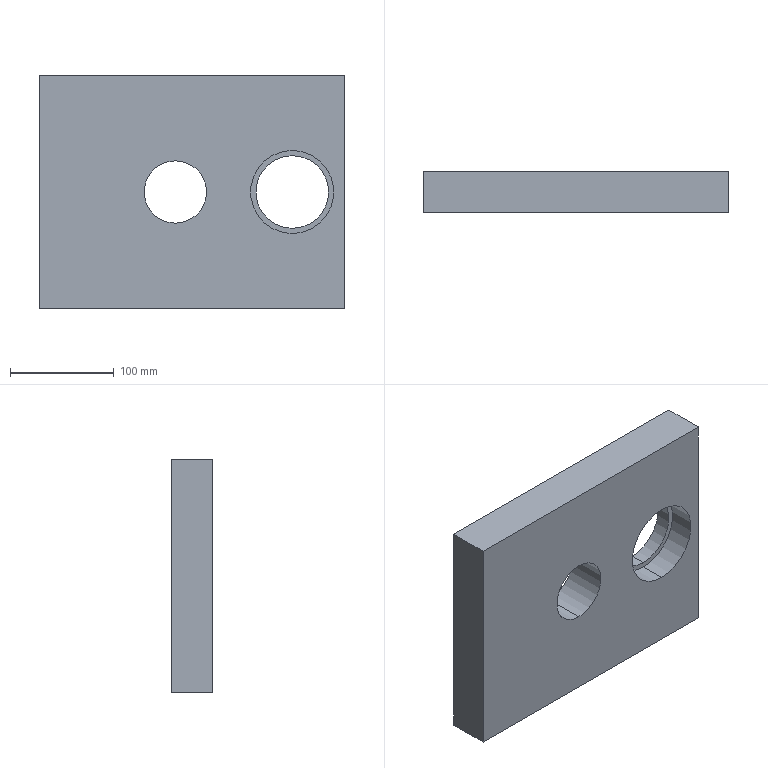Part | SolidWorks | features Cut 3, Extrusion 1 | 1 solid | 13 faces | box 293 x 40 x 225 mm | volume 2340512 mm3 | plane 7 | cylinder 6 | commonest cylinder face diameters 60 x2 70 x2 80 x2
STEP:
#1=CARTESIAN_POINT('',(96.5,40.,35.));
#2=VERTEX_POINT('',#1);
#3=CARTESIAN_POINT('',(96.5,40.,-35.));
#4=VERTEX_POINT('',#3);
#5=CARTESIAN_POINT('',(96.5,40.,0.));
#6=DIRECTION('',(0.,-1.,0.));
#7=DIRECTION('',(0.,0.,-1.));
#8=AXIS2_PLACEMENT_3D('',#5,#6,#7);
#9=CIRCLE('',#8,35.);
#10=EDGE_CURVE('',#2,#4,#9,.T.);
#11=ORIENTED_EDGE('',*,*,#10,.F.);
#12=CARTESIAN_POINT('',(96.5,25.,35.));
#13=VERTEX_POINT('',#12);
#14=CARTESIAN_POINT('',(96.5,40.,35.));
#15=DIRECTION('',(0.,-1.,0.));
#16=VECTOR('',#15,1000.);
#17=LINE('',#14,#16);
#18=EDGE_CURVE('',#2,#13,#17,.T.);
#19=ORIENTED_EDGE('',*,*,#18,.T.);
#20=CARTESIAN_POINT('',(96.5,25.,-35.));
#21=VERTEX_POINT('',#20);
#22=CARTESIAN_POINT('',(96.5,25.,0.));
#23=DIRECTION('',(0.,-1.,0.));
#24=DIRECTION('',(0.,0.,-1.));
#25=AXIS2_PLACEMENT_3D('',#22,#23,#24);
#26=CIRCLE('',#25,35.);
#27=EDGE_CURVE('',#13,#21,#26,.T.);
#28=ORIENTED_EDGE('',*,*,#27,.T.);
#29=CARTESIAN_POINT('',(96.5,40.,-35.));
#30=DIRECTION('',(0.,-1.,0.));
#31=VECTOR('',#30,1000.);
#32=LINE('',#29,#31);
#33=EDGE_CURVE('',#4,#21,#32,.T.);
#34=ORIENTED_EDGE('',*,*,#33,.F.);
#35=EDGE_LOOP('',(#11,#19,#28,#34));
#36=FACE_OUTER_BOUND('',#35,.T.);
#37=CARTESIAN_POINT('',(96.5,40.,0.));
#38=DIRECTION('',(0.,-1.,0.));
#39=DIRECTION('',(0.,0.,-1.));
#40=AXIS2_PLACEMENT_3D('',#37,#38,#39);
#41=CYLINDRICAL_SURFACE('',#40,35.);
#42=ADVANCED_FACE('',(#36),#41,.F.);
#43=CARTESIAN_POINT('',(-16.,40.,30.));
#44=VERTEX_POINT('',#43);
#45=CARTESIAN_POINT('',(-16.,40.,-30.));
#46=VERTEX_POINT('',#45);
#47=CARTESIAN_POINT('',(-16.,40.,0.));
#48=DIRECTION('',(0.,-1.,0.));
#49=DIRECTION('',(0.,0.,-1.));
#50=AXIS2_PLACEMENT_3D('',#47,#48,#49);
#51=CIRCLE('',#50,30.);
#52=EDGE_CURVE('',#44,#46,#51,.T.);
#53=ORIENTED_EDGE('',*,*,#52,.F.);
#54=CARTESIAN_POINT('',(-16.,0.,30.));
#55=VERTEX_POINT('',#54);
#56=CARTESIAN_POINT('',(-16.,40.,30.));
#57=DIRECTION('',(0.,-1.,0.));
#58=VECTOR('',#57,1000.);
#59=LINE('',#56,#58);
#60=EDGE_CURVE('',#44,#55,#59,.T.);
#61=ORIENTED_EDGE('',*,*,#60,.T.);
#62=CARTESIAN_POINT('',(-16.,0.,-30.));
#63=VERTEX_POINT('',#62);
#64=CARTESIAN_POINT('',(-16.,0.,0.));
#65=DIRECTION('',(0.,-1.,0.));
#66=DIRECTION('',(0.,0.,-1.));
#67=AXIS2_PLACEMENT_3D('',#64,#65,#66);
#68=CIRCLE('',#67,30.);
#69=EDGE_CURVE('',#55,#63,#68,.T.);
#70=ORIENTED_EDGE('',*,*,#69,.T.);
#71=CARTESIAN_POINT('',(-16.,40.,-30.));
#72=DIRECTION('',(0.,-1.,0.));
#73=VECTOR('',#72,1000.);
#74=LINE('',#71,#73);
#75=EDGE_CURVE('',#46,#63,#74,.T.);
#76=ORIENTED_EDGE('',*,*,#75,.F.);
#77=EDGE_LOOP('',(#53,#61,#70,#76));
#78=FACE_OUTER_BOUND('',#77,.T.);
#79=CARTESIAN_POINT('',(-16.,40.,0.));
#80=DIRECTION('',(0.,-1.,0.));
#81=DIRECTION('',(0.,0.,-1.));
#82=AXIS2_PLACEMENT_3D('',#79,#80,#81);
#83=CYLINDRICAL_SURFACE('',#82,30.);
#84=ADVANCED_FACE('',(#78),#83,.F.);
#85=CARTESIAN_POINT('',(96.5,25.,40.));
#86=VERTEX_POINT('',#85);
#87=CARTESIAN_POINT('',(96.5,25.,-40.));
#88=VERTEX_POINT('',#87);
#89=CARTESIAN_POINT('',(96.5,25.,0.));
#90=DIRECTION('',(0.,-1.,0.));
#91=DIRECTION('',(0.,0.,-1.));
#92=AXIS2_PLACEMENT_3D('',#89,#90,#91);
#93=CIRCLE('',#92,40.);
#94=EDGE_CURVE('',#86,#88,#93,.T.);
#95=ORIENTED_EDGE('',*,*,#94,.F.);
#96=CARTESIAN_POINT('',(96.5,0.,40.));
#97=VERTEX_POINT('',#96);
#98=CARTESIAN_POINT('',(96.5,25.,40.));
#99=DIRECTION('',(0.,-1.,0.));
#100=VECTOR('',#99,1000.);
#101=LINE('',#98,#100);
#102=EDGE_CURVE('',#86,#97,#101,.T.);
#103=ORIENTED_EDGE('',*,*,#102,.T.);
#104=CARTESIAN_POINT('',(96.5,0.,-40.));
#105=VERTEX_POINT('',#104);
#106=CARTESIAN_POINT('',(96.5,0.,0.));
#107=DIRECTION('',(0.,-1.,0.));
#108=DIRECTION('',(0.,0.,-1.));
#109=AXIS2_PLACEMENT_3D('',#106,#107,#108);
#110=CIRCLE('',#109,40.);
#111=EDGE_CURVE('',#97,#105,#110,.T.);
#112=ORIENTED_EDGE('',*,*,#111,.T.);
#113=CARTESIAN_POINT('',(96.5,25.,-40.));
#114=DIRECTION('',(0.,-1.,0.));
#115=VECTOR('',#114,1000.);
#116=LINE('',#113,#115);
#117=EDGE_CURVE('',#88,#105,#116,.T.);
#118=ORIENTED_EDGE('',*,*,#117,.F.);
#119=EDGE_LOOP('',(#95,#103,#112,#118));
#120=FACE_OUTER_BOUND('',#119,.T.);
#121=CARTESIAN_POINT('',(96.5,25.,0.));
#122=DIRECTION('',(0.,-1.,0.));
#123=DIRECTION('',(0.,0.,-1.));
#124=AXIS2_PLACEMENT_3D('',#121,#122,#123);
#125=CYLINDRICAL_SURFACE('',#124,40.);
#126=ADVANCED_FACE('',(#120),#125,.F.);
#127=CARTESIAN_POINT('',(146.5,0.,112.5));
#128=VERTEX_POINT('',#127);
#129=CARTESIAN_POINT('',(146.5,0.,-112.5));
#130=VERTEX_POINT('',#129);
#131=CARTESIAN_POINT('',(146.5,0.,112.5));
#132=DIRECTION('',(0.,0.,-1.));
#133=VECTOR('',#132,1000.);
#134=LINE('',#131,#133);
#135=EDGE_CURVE('',#128,#130,#134,.T.);
#136=ORIENTED_EDGE('',*,*,#135,.T.);
#137=CARTESIAN_POINT('',(146.5,40.,-112.5));
#138=VERTEX_POINT('',#137);
#139=CARTESIAN_POINT('',(146.5,40.,-112.5));
#140=DIRECTION('',(0.,-1.,0.));
#141=VECTOR('',#140,1000.);
#142=LINE('',#139,#141);
#143=EDGE_CURVE('',#138,#130,#142,.T.);
#144=ORIENTED_EDGE('',*,*,#143,.F.);
#145=CARTESIAN_POINT('',(146.5,40.,112.5));
#146=VERTEX_POINT('',#145);
#147=CARTESIAN_POINT('',(146.5,40.,112.5));
#148=DIRECTION('',(0.,0.,-1.));
#149=VECTOR('',#148,1000.);
#150=LINE('',#147,#149);
#151=EDGE_CURVE('',#146,#138,#150,.T.);
#152=ORIENTED_EDGE('',*,*,#151,.F.);
#153=CARTESIAN_POINT('',(146.5,40.,112.5));
#154=DIRECTION('',(0.,-1.,0.));
#155=VECTOR('',#154,1000.);
#156=LINE('',#153,#155);
#157=EDGE_CURVE('',#146,#128,#156,.T.);
#158=ORIENTED_EDGE('',*,*,#157,.T.);
#159=EDGE_LOOP('',(#136,#144,#152,#158));
#160=FACE_OUTER_BOUND('',#159,.T.);
#161=CARTESIAN_POINT('',(146.5,40.,112.5));
#162=DIRECTION('',(-1.,0.,0.));
#163=DIRECTION('',(0.,0.,1.));
#164=AXIS2_PLACEMENT_3D('',#161,#162,#163);
#165=PLANE('',#164);
#166=ADVANCED_FACE('',(#160),#165,.F.);
#167=CARTESIAN_POINT('',(-146.5,0.,-112.5));
#168=VERTEX_POINT('',#167);
#169=CARTESIAN_POINT('',(-146.5,0.,-112.5));
#170=DIRECTION('',(-1.,0.,0.));
#171=VECTOR('',#170,1000.);
#172=LINE('',#169,#171);
#173=EDGE_CURVE('',#130,#168,#172,.T.);
#174=ORIENTED_EDGE('',*,*,#173,.T.);
#175=CARTESIAN_POINT('',(-146.5,40.,-112.5));
#176=VERTEX_POINT('',#175);
#177=CARTESIAN_POINT('',(-146.5,40.,-112.5));
#178=DIRECTION('',(0.,-1.,0.));
#179=VECTOR('',#178,1000.);
#180=LINE('',#177,#179);
#181=EDGE_CURVE('',#176,#168,#180,.T.);
#182=ORIENTED_EDGE('',*,*,#181,.F.);
#183=CARTESIAN_POINT('',(-146.5,40.,-112.5));
#184=DIRECTION('',(-1.,0.,0.));
#185=VECTOR('',#184,1000.);
#186=LINE('',#183,#185);
#187=EDGE_CURVE('',#138,#176,#186,.T.);
#188=ORIENTED_EDGE('',*,*,#187,.F.);
#189=ORIENTED_EDGE('',*,*,#143,.T.);
#190=EDGE_LOOP('',(#174,#182,#188,#189));
#191=FACE_OUTER_BOUND('',#190,.T.);
#192=CARTESIAN_POINT('',(-146.5,40.,-112.5));
#193=DIRECTION('',(0.,0.,1.));
#194=DIRECTION('',(1.,0.,0.));
#195=AXIS2_PLACEMENT_3D('',#192,#193,#194);
#196=PLANE('',#195);
#197=ADVANCED_FACE('',(#191),#196,.F.);
#198=CARTESIAN_POINT('',(-146.5,0.,112.5));
#199=VERTEX_POINT('',#198);
#200=CARTESIAN_POINT('',(-146.5,0.,112.5));
#201=DIRECTION('',(0.,0.,1.));
#202=VECTOR('',#201,1000.);
#203=LINE('',#200,#202);
#204=EDGE_CURVE('',#168,#199,#203,.T.);
#205=ORIENTED_EDGE('',*,*,#204,.T.);
#206=CARTESIAN_POINT('',(-146.5,40.,112.5));
#207=VERTEX_POINT('',#206);
#208=CARTESIAN_POINT('',(-146.5,40.,112.5));
#209=DIRECTION('',(0.,-1.,0.));
#210=VECTOR('',#209,1000.);
#211=LINE('',#208,#210);
#212=EDGE_CURVE('',#207,#199,#211,.T.);
#213=ORIENTED_EDGE('',*,*,#212,.F.);
#214=CARTESIAN_POINT('',(-146.5,40.,112.5));
#215=DIRECTION('',(0.,0.,1.));
#216=VECTOR('',#215,1000.);
#217=LINE('',#214,#216);
#218=EDGE_CURVE('',#176,#207,#217,.T.);
#219=ORIENTED_EDGE('',*,*,#218,.F.);
#220=ORIENTED_EDGE('',*,*,#181,.T.);
#221=EDGE_LOOP('',(#205,#213,#219,#220));
#222=FACE_OUTER_BOUND('',#221,.T.);
#223=CARTESIAN_POINT('',(-146.5,40.,112.5));
#224=DIRECTION('',(1.,0.,0.));
#225=DIRECTION('',(0.,0.,-1.));
#226=AXIS2_PLACEMENT_3D('',#223,#224,#225);
#227=PLANE('',#226);
#228=ADVANCED_FACE('',(#222),#227,.F.);
#229=CARTESIAN_POINT('',(-146.5,0.,112.5));
#230=DIRECTION('',(1.,0.,0.));
#231=VECTOR('',#230,1000.);
#232=LINE('',#229,#231);
#233=EDGE_CURVE('',#199,#128,#232,.T.);
#234=ORIENTED_EDGE('',*,*,#233,.T.);
#235=ORIENTED_EDGE('',*,*,#157,.F.);
#236=CARTESIAN_POINT('',(-146.5,40.,112.5));
#237=DIRECTION('',(1.,0.,0.));
#238=VECTOR('',#237,1000.);
#239=LINE('',#236,#238);
#240=EDGE_CURVE('',#207,#146,#239,.T.);
#241=ORIENTED_EDGE('',*,*,#240,.F.);
#242=ORIENTED_EDGE('',*,*,#212,.T.);
#243=EDGE_LOOP('',(#234,#235,#241,#242));
#244=FACE_OUTER_BOUND('',#243,.T.);
#245=CARTESIAN_POINT('',(-146.5,40.,112.5));
#246=DIRECTION('',(0.,0.,-1.));
#247=DIRECTION('',(-1.,0.,0.));
#248=AXIS2_PLACEMENT_3D('',#245,#246,#247);
#249=PLANE('',#248);
#250=ADVANCED_FACE('',(#244),#249,.F.);
#251=CARTESIAN_POINT('',(96.5,40.,0.));
#252=DIRECTION('',(0.,-1.,0.));
#253=DIRECTION('',(0.,0.,-1.));
#254=AXIS2_PLACEMENT_3D('',#251,#252,#253);
#255=CIRCLE('',#254,35.);
#256=EDGE_CURVE('',#4,#2,#255,.T.);
#257=ORIENTED_EDGE('',*,*,#256,.T.);
#258=ORIENTED_EDGE('',*,*,#10,.T.);
#259=EDGE_LOOP('',(#257,#258));
#260=FACE_BOUND('',#259,.T.);
#261=CARTESIAN_POINT('',(-16.,40.,0.));
#262=DIRECTION('',(0.,-1.,0.));
#263=DIRECTION('',(0.,0.,-1.));
#264=AXIS2_PLACEMENT_3D('',#261,#262,#263);
#265=CIRCLE('',#264,30.);
#266=EDGE_CURVE('',#46,#44,#265,.T.);
#267=ORIENTED_EDGE('',*,*,#266,.T.);
#268=ORIENTED_EDGE('',*,*,#52,.T.);
#269=EDGE_LOOP('',(#267,#268));
#270=FACE_BOUND('',#269,.T.);
#271=ORIENTED_EDGE('',*,*,#151,.T.);
#272=ORIENTED_EDGE('',*,*,#187,.T.);
#273=ORIENTED_EDGE('',*,*,#218,.T.);
#274=ORIENTED_EDGE('',*,*,#240,.T.);
#275=EDGE_LOOP('',(#271,#272,#273,#274));
#276=FACE_OUTER_BOUND('',#275,.T.);
#277=CARTESIAN_POINT('',(0.,40.,0.));
#278=DIRECTION('',(0.,-1.,0.));
#279=DIRECTION('',(0.,0.,-1.));
#280=AXIS2_PLACEMENT_3D('',#277,#278,#279);
#281=PLANE('',#280);
#282=ADVANCED_FACE('',(#260,#270,#276),#281,.F.);
#283=CARTESIAN_POINT('',(-16.,0.,0.));
#284=DIRECTION('',(0.,-1.,0.));
#285=DIRECTION('',(0.,0.,-1.));
#286=AXIS2_PLACEMENT_3D('',#283,#284,#285);
#287=CIRCLE('',#286,30.);
#288=EDGE_CURVE('',#63,#55,#287,.T.);
#289=ORIENTED_EDGE('',*,*,#288,.F.);
#290=ORIENTED_EDGE('',*,*,#69,.F.);
#291=EDGE_LOOP('',(#289,#290));
#292=FACE_BOUND('',#291,.T.);
#293=CARTESIAN_POINT('',(96.5,0.,0.));
#294=DIRECTION('',(0.,-1.,0.));
#295=DIRECTION('',(0.,0.,-1.));
#296=AXIS2_PLACEMENT_3D('',#293,#294,#295);
#297=CIRCLE('',#296,40.);
#298=EDGE_CURVE('',#105,#97,#297,.T.);
#299=ORIENTED_EDGE('',*,*,#298,.F.);
#300=ORIENTED_EDGE('',*,*,#111,.F.);
#301=EDGE_LOOP('',(#299,#300));
#302=FACE_BOUND('',#301,.T.);
#303=ORIENTED_EDGE('',*,*,#135,.F.);
#304=ORIENTED_EDGE('',*,*,#233,.F.);
#305=ORIENTED_EDGE('',*,*,#204,.F.);
#306=ORIENTED_EDGE('',*,*,#173,.F.);
#307=EDGE_LOOP('',(#303,#304,#305,#306));
#308=FACE_OUTER_BOUND('',#307,.T.);
#309=CARTESIAN_POINT('',(0.,0.,0.));
#310=DIRECTION('',(0.,-1.,0.));
#311=DIRECTION('',(0.,0.,-1.));
#312=AXIS2_PLACEMENT_3D('',#309,#310,#311);
#313=PLANE('',#312);
#314=ADVANCED_FACE('',(#292,#302,#308),#313,.T.);
#315=ORIENTED_EDGE('',*,*,#102,.F.);
#316=CARTESIAN_POINT('',(96.5,25.,0.));
#317=DIRECTION('',(0.,-1.,0.));
#318=DIRECTION('',(0.,0.,-1.));
#319=AXIS2_PLACEMENT_3D('',#316,#317,#318);
#320=CIRCLE('',#319,40.);
#321=EDGE_CURVE('',#88,#86,#320,.T.);
#322=ORIENTED_EDGE('',*,*,#321,.F.);
#323=ORIENTED_EDGE('',*,*,#117,.T.);
#324=ORIENTED_EDGE('',*,*,#298,.T.);
#325=EDGE_LOOP('',(#315,#322,#323,#324));
#326=FACE_OUTER_BOUND('',#325,.T.);
#327=CARTESIAN_POINT('',(96.5,25.,0.));
#328=DIRECTION('',(0.,-1.,0.));
#329=DIRECTION('',(0.,0.,-1.));
#330=AXIS2_PLACEMENT_3D('',#327,#328,#329);
#331=CYLINDRICAL_SURFACE('',#330,40.);
#332=ADVANCED_FACE('',(#326),#331,.F.);
#333=CARTESIAN_POINT('',(96.5,25.,0.));
#334=DIRECTION('',(0.,-1.,0.));
#335=DIRECTION('',(0.,0.,-1.));
#336=AXIS2_PLACEMENT_3D('',#333,#334,#335);
#337=CIRCLE('',#336,35.);
#338=EDGE_CURVE('',#21,#13,#337,.T.);
#339=ORIENTED_EDGE('',*,*,#338,.F.);
#340=ORIENTED_EDGE('',*,*,#27,.F.);
#341=EDGE_LOOP('',(#339,#340));
#342=FACE_BOUND('',#341,.T.);
#343=ORIENTED_EDGE('',*,*,#321,.T.);
#344=ORIENTED_EDGE('',*,*,#94,.T.);
#345=EDGE_LOOP('',(#343,#344));
#346=FACE_OUTER_BOUND('',#345,.T.);
#347=CARTESIAN_POINT('',(96.5,25.,0.));
#348=DIRECTION('',(0.,-1.,0.));
#349=DIRECTION('',(0.,0.,-1.));
#350=AXIS2_PLACEMENT_3D('',#347,#348,#349);
#351=PLANE('',#350);
#352=ADVANCED_FACE('',(#342,#346),#351,.T.);
#353=ORIENTED_EDGE('',*,*,#60,.F.);
#354=ORIENTED_EDGE('',*,*,#266,.F.);
#355=ORIENTED_EDGE('',*,*,#75,.T.);
#356=ORIENTED_EDGE('',*,*,#288,.T.);
#357=EDGE_LOOP('',(#353,#354,#355,#356));
#358=FACE_OUTER_BOUND('',#357,.T.);
#359=CARTESIAN_POINT('',(-16.,40.,0.));
#360=DIRECTION('',(0.,-1.,0.));
#361=DIRECTION('',(0.,0.,-1.));
#362=AXIS2_PLACEMENT_3D('',#359,#360,#361);
#363=CYLINDRICAL_SURFACE('',#362,30.);
#364=ADVANCED_FACE('',(#358),#363,.F.);
#365=ORIENTED_EDGE('',*,*,#18,.F.);
#366=ORIENTED_EDGE('',*,*,#256,.F.);
#367=ORIENTED_EDGE('',*,*,#33,.T.);
#368=ORIENTED_EDGE('',*,*,#338,.T.);
#369=EDGE_LOOP('',(#365,#366,#367,#368));
#370=FACE_OUTER_BOUND('',#369,.T.);
#371=CARTESIAN_POINT('',(96.5,40.,0.));
#372=DIRECTION('',(0.,-1.,0.));
#373=DIRECTION('',(0.,0.,-1.));
#374=AXIS2_PLACEMENT_3D('',#371,#372,#373);
#375=CYLINDRICAL_SURFACE('',#374,35.);
#376=ADVANCED_FACE('',(#370),#375,.F.);
#377=CLOSED_SHELL('',(#42,#84,#126,#166,#197,#228,#250,#282,#314,#332,#352,#364,#376));
#378=MANIFOLD_SOLID_BREP('',#377);
#379=CARTESIAN_POINT('',(0.,0.,0.));
#380=DIRECTION('',(0.,0.,1.));
#381=DIRECTION('',(1.,0.,0.));
#382=AXIS2_PLACEMENT_3D('',#379,#380,#381);
#383=(LENGTH_UNIT()NAMED_UNIT(*)SI_UNIT(.MILLI.,.METRE.));
#384=UNCERTAINTY_MEASURE_WITH_UNIT(LENGTH_MEASURE(0.00001),#383,'','');
#385=(NAMED_UNIT(*)PLANE_ANGLE_UNIT()SI_UNIT($,.RADIAN.));
#386=(NAMED_UNIT(*)SI_UNIT($,.STERADIAN.)SOLID_ANGLE_UNIT());
#387=(GEOMETRIC_REPRESENTATION_CONTEXT(3)GLOBAL_UNCERTAINTY_ASSIGNED_CONTEXT((#384))GLOBAL_UNIT_ASSIGNED_CONTEXT((#383,#385,#386))REPRESENTATION_CONTEXT('',''));
#388=ADVANCED_BREP_SHAPE_REPRESENTATION('',(#378,#382),#387);